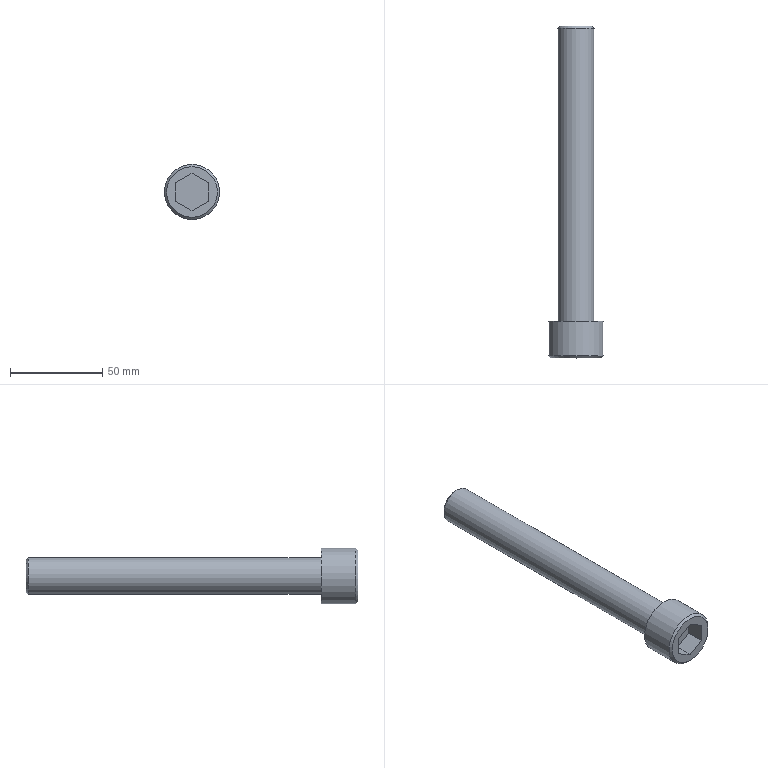Part | STEP file | M20.00-160.00 | 1 solid | 14 faces | box 30 x 180 x 30 mm | volume 61632 mm3 | plane 10 | cylinder 2 | cone 2 | commonest cylinder face diameters 20 x1 30 x1